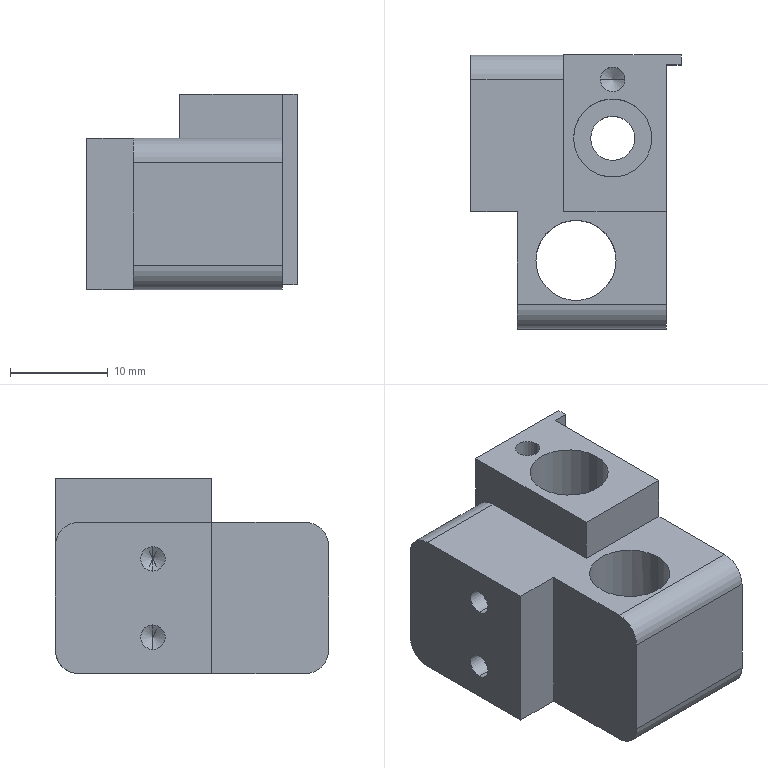Part | NX | features BREP 1 | 1 solid | 46 faces | box 21.5 x 28 x 20 mm | volume 6689 mm3 | cylinder 22 | plane 14 | cone 10 | commonest cylinder face diameters 2.5 x6 2.05 x4 5 x4 3.3 x2 4.5 x2 8 x2
STEP:
#1=CARTESIAN_POINT('',(20.,-9.5,15.5));
#2=VERTEX_POINT('',#1);
#3=CARTESIAN_POINT('',(20.,-12.,13.));
#4=VERTEX_POINT('',#3);
#5=CARTESIAN_POINT('',(20.,-9.5,13.));
#6=DIRECTION('',(1.,0.,0.));
#7=DIRECTION('',(0.,-1.,0.));
#8=AXIS2_PLACEMENT_3D('',#5,#6,#7);
#9=CIRCLE('',#8,2.5);
#10=EDGE_CURVE('',#2,#4,#9,.T.);
#11=ORIENTED_EDGE('',*,*,#10,.F.);
#12=CARTESIAN_POINT('',(4.75,-9.5,15.5));
#13=VERTEX_POINT('',#12);
#14=CARTESIAN_POINT('',(20.,-9.5,15.5));
#15=DIRECTION('',(1.,0.,0.));
#16=VECTOR('',#15,1000.);
#17=LINE('',#14,#16);
#18=EDGE_CURVE('',#13,#2,#17,.T.);
#19=ORIENTED_EDGE('',*,*,#18,.F.);
#20=CARTESIAN_POINT('',(4.75,-12.,13.));
#21=VERTEX_POINT('',#20);
#22=CARTESIAN_POINT('',(4.75,-9.5,13.));
#23=DIRECTION('',(-1.,0.,0.));
#24=DIRECTION('',(0.,0.,-1.));
#25=AXIS2_PLACEMENT_3D('',#22,#23,#24);
#26=CIRCLE('',#25,2.5);
#27=EDGE_CURVE('',#21,#13,#26,.T.);
#28=ORIENTED_EDGE('',*,*,#27,.F.);
#29=CARTESIAN_POINT('',(4.75,-12.,13.));
#30=DIRECTION('',(-1.,0.,0.));
#31=VECTOR('',#30,1000.);
#32=LINE('',#29,#31);
#33=EDGE_CURVE('',#4,#21,#32,.T.);
#34=ORIENTED_EDGE('',*,*,#33,.F.);
#35=EDGE_LOOP('',(#11,#19,#28,#34));
#36=FACE_BOUND('',#35,.T.);
#37=CARTESIAN_POINT('',(0.,-9.5,13.));
#38=DIRECTION('',(1.,0.,0.));
#39=DIRECTION('',(0.,1.,0.));
#40=AXIS2_PLACEMENT_3D('',#37,#38,#39);
#41=CYLINDRICAL_SURFACE('',#40,2.5);
#42=ADVANCED_FACE('',(#36),#41,.T.);
#43=CARTESIAN_POINT('',(4.75,-9.5,0.));
#44=VERTEX_POINT('',#43);
#45=CARTESIAN_POINT('',(4.75,-12.,2.5));
#46=VERTEX_POINT('',#45);
#47=CARTESIAN_POINT('',(4.75,-9.5,2.5));
#48=DIRECTION('',(-1.,0.,0.));
#49=DIRECTION('',(0.,0.,-1.));
#50=AXIS2_PLACEMENT_3D('',#47,#48,#49);
#51=CIRCLE('',#50,2.5);
#52=EDGE_CURVE('',#44,#46,#51,.T.);
#53=ORIENTED_EDGE('',*,*,#52,.F.);
#54=CARTESIAN_POINT('',(20.,-9.5,0.));
#55=VERTEX_POINT('',#54);
#56=CARTESIAN_POINT('',(0.,-9.5,0.));
#57=DIRECTION('',(-1.,0.,0.));
#58=VECTOR('',#57,1000.);
#59=LINE('',#56,#58);
#60=EDGE_CURVE('',#55,#44,#59,.T.);
#61=ORIENTED_EDGE('',*,*,#60,.F.);
#62=CARTESIAN_POINT('',(20.,-12.,2.5));
#63=VERTEX_POINT('',#62);
#64=CARTESIAN_POINT('',(20.,-9.5,2.5));
#65=DIRECTION('',(1.,0.,0.));
#66=DIRECTION('',(0.,-1.,0.));
#67=AXIS2_PLACEMENT_3D('',#64,#65,#66);
#68=CIRCLE('',#67,2.5);
#69=EDGE_CURVE('',#63,#55,#68,.T.);
#70=ORIENTED_EDGE('',*,*,#69,.F.);
#71=CARTESIAN_POINT('',(0.,-12.,2.5));
#72=DIRECTION('',(1.,0.,0.));
#73=VECTOR('',#72,1000.);
#74=LINE('',#71,#73);
#75=EDGE_CURVE('',#46,#63,#74,.T.);
#76=ORIENTED_EDGE('',*,*,#75,.F.);
#77=EDGE_LOOP('',(#53,#61,#70,#76));
#78=FACE_BOUND('',#77,.T.);
#79=CARTESIAN_POINT('',(0.,-9.5,2.5));
#80=DIRECTION('',(1.,0.,0.));
#81=DIRECTION('',(0.,1.,0.));
#82=AXIS2_PLACEMENT_3D('',#79,#80,#81);
#83=CYLINDRICAL_SURFACE('',#82,2.5);
#84=ADVANCED_FACE('',(#78),#83,.T.);
#85=CARTESIAN_POINT('',(14.85,-5.,9.65));
#86=VERTEX_POINT('',#85);
#87=CARTESIAN_POINT('',(20.,-5.,9.65));
#88=VERTEX_POINT('',#87);
#89=CARTESIAN_POINT('',(20.,-5.,9.65));
#90=DIRECTION('',(1.,0.,0.));
#91=VECTOR('',#90,1000.);
#92=LINE('',#89,#91);
#93=EDGE_CURVE('',#86,#88,#92,.T.);
#94=ORIENTED_EDGE('',*,*,#93,.F.);
#95=CARTESIAN_POINT('',(14.85,-5.,6.35));
#96=VERTEX_POINT('',#95);
#97=CARTESIAN_POINT('',(14.85,-5.,9.65));
#98=CARTESIAN_POINT('',(14.85,-4.793,9.65));
#99=CARTESIAN_POINT('',(14.815,-4.417,9.563));
#100=CARTESIAN_POINT('',(14.759,-4.135,9.414));
#101=CARTESIAN_POINT('',(14.697,-3.881,9.229));
#102=CARTESIAN_POINT('',(14.635,-3.689,9.006));
#103=CARTESIAN_POINT('',(14.609,-3.615,8.902));
#104=CARTESIAN_POINT('',(14.529,-3.402,8.528));
#105=CARTESIAN_POINT('',(14.486,-3.315,7.999));
#106=CARTESIAN_POINT('',(14.529,-3.403,7.471));
#107=CARTESIAN_POINT('',(14.609,-3.614,7.099));
#108=CARTESIAN_POINT('',(14.636,-3.69,6.992));
#109=CARTESIAN_POINT('',(14.696,-3.878,6.774));
#110=CARTESIAN_POINT('',(14.759,-4.135,6.586));
#111=CARTESIAN_POINT('',(14.815,-4.415,6.438));
#112=CARTESIAN_POINT('',(14.85,-4.793,6.35));
#113=CARTESIAN_POINT('',(14.85,-5.,6.35));
#114=B_SPLINE_CURVE_WITH_KNOTS('',3,(#97,#98,#99,#100,#101,#102,#103,#104,#105,#106,#107,#108,#109,#110,#111,#112,#113),.UNSPECIFIED.,.F.,.F.,(4,1,1,1,1,1,1,1,1,1,1,1,1,1,4),(0.,0.125,0.1875,0.25,0.2812,0.3125,0.375,0.5,0.625,0.6875,0.7188,0.75,0.8125,0.875,1.),.UNSPECIFIED.);
#115=EDGE_CURVE('',#96,#86,#114,.F.);
#116=ORIENTED_EDGE('',*,*,#115,.F.);
#117=CARTESIAN_POINT('',(20.,-5.,6.35));
#118=VERTEX_POINT('',#117);
#119=CARTESIAN_POINT('',(20.,-5.,6.35));
#120=DIRECTION('',(1.,0.,0.));
#121=VECTOR('',#120,1000.);
#122=LINE('',#119,#121);
#123=EDGE_CURVE('',#96,#118,#122,.T.);
#124=ORIENTED_EDGE('',*,*,#123,.T.);
#125=CARTESIAN_POINT('',(20.,-5.,8.));
#126=DIRECTION('',(1.,0.,0.));
#127=DIRECTION('',(0.,0.,-1.));
#128=AXIS2_PLACEMENT_3D('',#125,#126,#127);
#129=CIRCLE('',#128,1.65);
#130=EDGE_CURVE('',#118,#88,#129,.T.);
#131=ORIENTED_EDGE('',*,*,#130,.T.);
#132=EDGE_LOOP('',(#94,#116,#124,#131));
#133=FACE_BOUND('',#132,.T.);
#134=CARTESIAN_POINT('',(20.,-5.,8.));
#135=DIRECTION('',(1.,0.,0.));
#136=DIRECTION('',(0.,0.,-1.));
#137=AXIS2_PLACEMENT_3D('',#134,#135,#136);
#138=CYLINDRICAL_SURFACE('',#137,1.65);
#139=ADVANCED_FACE('',(#133),#138,.F.);
#140=CARTESIAN_POINT('',(6.65,-5.,15.5));
#141=VERTEX_POINT('',#140);
#142=CARTESIAN_POINT('',(6.65,-5.,0.));
#143=VERTEX_POINT('',#142);
#144=CARTESIAN_POINT('',(6.65,-5.,15.5));
#145=DIRECTION('',(0.,0.,1.));
#146=VECTOR('',#145,1000.);
#147=LINE('',#144,#146);
#148=EDGE_CURVE('',#141,#143,#147,.F.);
#149=ORIENTED_EDGE('',*,*,#148,.T.);
#150=CARTESIAN_POINT('',(14.85,-5.,0.));
#151=VERTEX_POINT('',#150);
#152=CARTESIAN_POINT('',(10.75,-5.,0.));
#153=DIRECTION('',(0.,0.,1.));
#154=DIRECTION('',(1.,0.,0.));
#155=AXIS2_PLACEMENT_3D('',#152,#153,#154);
#156=CIRCLE('',#155,4.1);
#157=EDGE_CURVE('',#151,#143,#156,.T.);
#158=ORIENTED_EDGE('',*,*,#157,.F.);
#159=CARTESIAN_POINT('',(14.85,-5.,15.5));
#160=DIRECTION('',(0.,0.,1.));
#161=VECTOR('',#160,1000.);
#162=LINE('',#159,#161);
#163=EDGE_CURVE('',#151,#96,#162,.T.);
#164=ORIENTED_EDGE('',*,*,#163,.T.);
#165=ORIENTED_EDGE('',*,*,#115,.T.);
#166=CARTESIAN_POINT('',(14.85,-5.,15.5));
#167=VERTEX_POINT('',#166);
#168=CARTESIAN_POINT('',(14.85,-5.,15.5));
#169=DIRECTION('',(0.,0.,1.));
#170=VECTOR('',#169,1000.);
#171=LINE('',#168,#170);
#172=EDGE_CURVE('',#167,#86,#171,.F.);
#173=ORIENTED_EDGE('',*,*,#172,.F.);
#174=CARTESIAN_POINT('',(10.75,-5.,15.5));
#175=DIRECTION('',(0.,0.,1.));
#176=DIRECTION('',(1.,0.,0.));
#177=AXIS2_PLACEMENT_3D('',#174,#175,#176);
#178=CIRCLE('',#177,4.1);
#179=EDGE_CURVE('',#167,#141,#178,.T.);
#180=ORIENTED_EDGE('',*,*,#179,.T.);
#181=EDGE_LOOP('',(#149,#158,#164,#165,#173,#180));
#182=FACE_BOUND('',#181,.T.);
#183=CARTESIAN_POINT('',(10.75,-5.,15.5));
#184=DIRECTION('',(0.,0.,1.));
#185=DIRECTION('',(1.,0.,0.));
#186=AXIS2_PLACEMENT_3D('',#183,#184,#185);
#187=CYLINDRICAL_SURFACE('',#186,4.1);
#188=ADVANCED_FACE('',(#182),#187,.F.);
#189=CARTESIAN_POINT('',(4.75,-12.,0.));
#190=DIRECTION('',(0.,0.,-1.));
#191=VECTOR('',#190,1000.);
#192=LINE('',#189,#191);
#193=EDGE_CURVE('',#21,#46,#192,.T.);
#194=ORIENTED_EDGE('',*,*,#193,.T.);
#195=ORIENTED_EDGE('',*,*,#75,.T.);
#196=CARTESIAN_POINT('',(20.,-12.,0.));
#197=DIRECTION('',(0.,0.,1.));
#198=VECTOR('',#197,1000.);
#199=LINE('',#196,#198);
#200=EDGE_CURVE('',#63,#4,#199,.T.);
#201=ORIENTED_EDGE('',*,*,#200,.T.);
#202=ORIENTED_EDGE('',*,*,#33,.T.);
#203=EDGE_LOOP('',(#194,#195,#201,#202));
#204=FACE_BOUND('',#203,.T.);
#205=CARTESIAN_POINT('',(0.,-12.,0.));
#206=DIRECTION('',(0.,-1.,0.));
#207=DIRECTION('',(1.,0.,0.));
#208=AXIS2_PLACEMENT_3D('',#205,#206,#207);
#209=PLANE('',#208);
#210=ADVANCED_FACE('',(#204),#209,.T.);
#211=CARTESIAN_POINT('',(4.75,0.,0.));
#212=VERTEX_POINT('',#211);
#213=CARTESIAN_POINT('',(4.75,-12.,0.));
#214=DIRECTION('',(0.,1.,0.));
#215=VECTOR('',#214,1000.);
#216=LINE('',#213,#215);
#217=EDGE_CURVE('',#44,#212,#216,.T.);
#218=ORIENTED_EDGE('',*,*,#217,.F.);
#219=ORIENTED_EDGE('',*,*,#52,.T.);
#220=ORIENTED_EDGE('',*,*,#193,.F.);
#221=ORIENTED_EDGE('',*,*,#27,.T.);
#222=CARTESIAN_POINT('',(4.75,0.,15.5));
#223=VERTEX_POINT('',#222);
#224=CARTESIAN_POINT('',(4.75,-12.,15.5));
#225=DIRECTION('',(0.,1.,0.));
#226=VECTOR('',#225,1000.);
#227=LINE('',#224,#226);
#228=EDGE_CURVE('',#13,#223,#227,.T.);
#229=ORIENTED_EDGE('',*,*,#228,.T.);
#230=CARTESIAN_POINT('',(4.75,0.,0.));
#231=DIRECTION('',(0.,0.,-1.));
#232=VECTOR('',#231,1000.);
#233=LINE('',#230,#232);
#234=EDGE_CURVE('',#223,#212,#233,.T.);
#235=ORIENTED_EDGE('',*,*,#234,.T.);
#236=EDGE_LOOP('',(#218,#219,#220,#221,#229,#235));
#237=FACE_BOUND('',#236,.T.);
#238=CARTESIAN_POINT('',(4.75,-12.,0.));
#239=DIRECTION('',(1.,0.,0.));
#240=DIRECTION('',(0.,0.,-1.));
#241=AXIS2_PLACEMENT_3D('',#238,#239,#240);
#242=PLANE('',#241);
#243=ADVANCED_FACE('',(#237),#242,.F.);
#244=CARTESIAN_POINT('',(9.5,16.,13.));
#245=VERTEX_POINT('',#244);
#246=CARTESIAN_POINT('',(9.5,13.5,15.5));
#247=VERTEX_POINT('',#246);
#248=CARTESIAN_POINT('',(9.5,13.5,13.));
#249=DIRECTION('',(1.,0.,0.));
#250=DIRECTION('',(0.,0.,-1.));
#251=AXIS2_PLACEMENT_3D('',#248,#249,#250);
#252=CIRCLE('',#251,2.5);
#253=EDGE_CURVE('',#245,#247,#252,.T.);
#254=ORIENTED_EDGE('',*,*,#253,.F.);
#255=CARTESIAN_POINT('',(0.,16.,13.));
#256=VERTEX_POINT('',#255);
#257=CARTESIAN_POINT('',(0.,16.,13.));
#258=DIRECTION('',(1.,0.,0.));
#259=VECTOR('',#258,1000.);
#260=LINE('',#257,#259);
#261=EDGE_CURVE('',#256,#245,#260,.T.);
#262=ORIENTED_EDGE('',*,*,#261,.F.);
#263=CARTESIAN_POINT('',(0.,13.5,15.5));
#264=VERTEX_POINT('',#263);
#265=CARTESIAN_POINT('',(0.,13.5,13.));
#266=DIRECTION('',(-1.,0.,0.));
#267=DIRECTION('',(0.,0.,-1.));
#268=AXIS2_PLACEMENT_3D('',#265,#266,#267);
#269=CIRCLE('',#268,2.5);
#270=EDGE_CURVE('',#264,#256,#269,.T.);
#271=ORIENTED_EDGE('',*,*,#270,.F.);
#272=CARTESIAN_POINT('',(0.,13.5,15.5));
#273=DIRECTION('',(-1.,0.,0.));
#274=VECTOR('',#273,1000.);
#275=LINE('',#272,#274);
#276=EDGE_CURVE('',#247,#264,#275,.T.);
#277=ORIENTED_EDGE('',*,*,#276,.F.);
#278=EDGE_LOOP('',(#254,#262,#271,#277));
#279=FACE_BOUND('',#278,.T.);
#280=CARTESIAN_POINT('',(0.,13.5,13.));
#281=DIRECTION('',(-1.,0.,0.));
#282=DIRECTION('',(0.,0.,1.));
#283=AXIS2_PLACEMENT_3D('',#280,#281,#282);
#284=CYLINDRICAL_SURFACE('',#283,2.5);
#285=ADVANCED_FACE('',(#279),#284,.T.);
#286=CARTESIAN_POINT('',(20.,13.5,0.));
#287=VERTEX_POINT('',#286);
#288=CARTESIAN_POINT('',(20.,15.,0.5));
#289=VERTEX_POINT('',#288);
#290=CARTESIAN_POINT('',(20.,13.5,2.5));
#291=DIRECTION('',(1.,0.,0.));
#292=DIRECTION('',(0.,-1.,0.));
#293=AXIS2_PLACEMENT_3D('',#290,#291,#292);
#294=CIRCLE('',#293,2.5);
#295=EDGE_CURVE('',#287,#289,#294,.T.);
#296=ORIENTED_EDGE('',*,*,#295,.F.);
#297=CARTESIAN_POINT('',(0.,13.5,0.));
#298=VERTEX_POINT('',#297);
#299=CARTESIAN_POINT('',(21.5,13.5,0.));
#300=DIRECTION('',(1.,0.,0.));
#301=VECTOR('',#300,1000.);
#302=LINE('',#299,#301);
#303=EDGE_CURVE('',#298,#287,#302,.T.);
#304=ORIENTED_EDGE('',*,*,#303,.F.);
#305=CARTESIAN_POINT('',(0.,16.,2.5));
#306=VERTEX_POINT('',#305);
#307=CARTESIAN_POINT('',(0.,13.5,2.5));
#308=DIRECTION('',(-1.,0.,0.));
#309=DIRECTION('',(0.,0.,-1.));
#310=AXIS2_PLACEMENT_3D('',#307,#308,#309);
#311=CIRCLE('',#310,2.5);
#312=EDGE_CURVE('',#306,#298,#311,.T.);
#313=ORIENTED_EDGE('',*,*,#312,.F.);
#314=CARTESIAN_POINT('',(21.5,16.,2.5));
#315=VERTEX_POINT('',#314);
#316=CARTESIAN_POINT('',(0.,16.,2.5));
#317=DIRECTION('',(-1.,0.,0.));
#318=VECTOR('',#317,1000.);
#319=LINE('',#316,#318);
#320=EDGE_CURVE('',#315,#306,#319,.T.);
#321=ORIENTED_EDGE('',*,*,#320,.F.);
#322=CARTESIAN_POINT('',(21.5,15.,0.5));
#323=VERTEX_POINT('',#322);
#324=CARTESIAN_POINT('',(21.5,13.5,2.5));
#325=DIRECTION('',(1.,0.,0.));
#326=DIRECTION('',(0.,0.,1.));
#327=AXIS2_PLACEMENT_3D('',#324,#325,#326);
#328=CIRCLE('',#327,2.5);
#329=EDGE_CURVE('',#323,#315,#328,.T.);
#330=ORIENTED_EDGE('',*,*,#329,.F.);
#331=CARTESIAN_POINT('',(20.,15.,0.5));
#332=DIRECTION('',(1.,0.,0.));
#333=VECTOR('',#332,1000.);
#334=LINE('',#331,#333);
#335=EDGE_CURVE('',#289,#323,#334,.T.);
#336=ORIENTED_EDGE('',*,*,#335,.F.);
#337=EDGE_LOOP('',(#296,#304,#313,#321,#330,#336));
#338=FACE_BOUND('',#337,.T.);
#339=CARTESIAN_POINT('',(0.,13.5,2.5));
#340=DIRECTION('',(1.,0.,0.));
#341=DIRECTION('',(0.,0.,-1.));
#342=AXIS2_PLACEMENT_3D('',#339,#340,#341);
#343=CYLINDRICAL_SURFACE('',#342,2.5);
#344=ADVANCED_FACE('',(#338),#343,.T.);
#345=ORIENTED_EDGE('',*,*,#228,.F.);
#346=ORIENTED_EDGE('',*,*,#18,.T.);
#347=CARTESIAN_POINT('',(20.,0.,15.5));
#348=VERTEX_POINT('',#347);
#349=CARTESIAN_POINT('',(20.,-12.,15.5));
#350=DIRECTION('',(0.,1.,0.));
#351=VECTOR('',#350,1000.);
#352=LINE('',#349,#351);
#353=EDGE_CURVE('',#2,#348,#352,.T.);
#354=ORIENTED_EDGE('',*,*,#353,.T.);
#355=CARTESIAN_POINT('',(9.5,0.,15.5));
#356=VERTEX_POINT('',#355);
#357=CARTESIAN_POINT('',(20.,0.,15.5));
#358=DIRECTION('',(-1.,0.,0.));
#359=VECTOR('',#358,1000.);
#360=LINE('',#357,#359);
#361=EDGE_CURVE('',#348,#356,#360,.T.);
#362=ORIENTED_EDGE('',*,*,#361,.T.);
#363=CARTESIAN_POINT('',(9.5,0.,15.5));
#364=DIRECTION('',(0.,1.,0.));
#365=VECTOR('',#364,1000.);
#366=LINE('',#363,#365);
#367=EDGE_CURVE('',#356,#247,#366,.T.);
#368=ORIENTED_EDGE('',*,*,#367,.T.);
#369=ORIENTED_EDGE('',*,*,#276,.T.);
#370=CARTESIAN_POINT('',(0.,0.,15.5));
#371=VERTEX_POINT('',#370);
#372=CARTESIAN_POINT('',(0.,0.,15.5));
#373=DIRECTION('',(0.,-1.,0.));
#374=VECTOR('',#373,1000.);
#375=LINE('',#372,#374);
#376=EDGE_CURVE('',#264,#371,#375,.T.);
#377=ORIENTED_EDGE('',*,*,#376,.T.);
#378=CARTESIAN_POINT('',(0.,0.,15.5));
#379=DIRECTION('',(1.,0.,0.));
#380=VECTOR('',#379,1000.);
#381=LINE('',#378,#380);
#382=EDGE_CURVE('',#371,#223,#381,.T.);
#383=ORIENTED_EDGE('',*,*,#382,.T.);
#384=EDGE_LOOP('',(#345,#346,#354,#362,#368,#369,#377,#383));
#385=FACE_BOUND('',#384,.T.);
#386=ORIENTED_EDGE('',*,*,#179,.F.);
#387=CARTESIAN_POINT('',(10.75,-5.,15.5));
#388=DIRECTION('',(0.,0.,1.));
#389=DIRECTION('',(1.,0.,0.));
#390=AXIS2_PLACEMENT_3D('',#387,#388,#389);
#391=CIRCLE('',#390,4.1);
#392=EDGE_CURVE('',#141,#167,#391,.T.);
#393=ORIENTED_EDGE('',*,*,#392,.F.);
#394=EDGE_LOOP('',(#386,#393));
#395=FACE_BOUND('',#394,.T.);
#396=CARTESIAN_POINT('',(0.,0.,15.5));
#397=DIRECTION('',(0.,0.,-1.));
#398=DIRECTION('',(-1.,0.,0.));
#399=AXIS2_PLACEMENT_3D('',#396,#397,#398);
#400=PLANE('',#399);
#401=ADVANCED_FACE('',(#385,#395),#400,.F.);
#402=CARTESIAN_POINT('',(9.5,0.,20.));
#403=VERTEX_POINT('',#402);
#404=CARTESIAN_POINT('',(9.5,16.,20.));
#405=VERTEX_POINT('',#404);
#406=CARTESIAN_POINT('',(9.5,0.,20.));
#407=DIRECTION('',(0.,1.,0.));
#408=VECTOR('',#407,1000.);
#409=LINE('',#406,#408);
#410=EDGE_CURVE('',#403,#405,#409,.T.);
#411=ORIENTED_EDGE('',*,*,#410,.T.);
#412=CARTESIAN_POINT('',(9.5,16.,15.5));
#413=DIRECTION('',(0.,0.,1.));
#414=VECTOR('',#413,1000.);
#415=LINE('',#412,#414);
#416=EDGE_CURVE('',#245,#405,#415,.T.);
#417=ORIENTED_EDGE('',*,*,#416,.F.);
#418=ORIENTED_EDGE('',*,*,#253,.T.);
#419=ORIENTED_EDGE('',*,*,#367,.F.);
#420=CARTESIAN_POINT('',(9.5,0.,15.5));
#421=DIRECTION('',(0.,0.,1.));
#422=VECTOR('',#421,1000.);
#423=LINE('',#420,#422);
#424=EDGE_CURVE('',#356,#403,#423,.T.);
#425=ORIENTED_EDGE('',*,*,#424,.T.);
#426=EDGE_LOOP('',(#411,#417,#418,#419,#425));
#427=FACE_BOUND('',#426,.T.);
#428=CARTESIAN_POINT('',(9.5,0.,15.5));
#429=DIRECTION('',(1.,0.,0.));
#430=DIRECTION('',(0.,0.,-1.));
#431=AXIS2_PLACEMENT_3D('',#428,#429,#430);
#432=PLANE('',#431);
#433=ADVANCED_FACE('',(#427),#432,.F.);
#434=CARTESIAN_POINT('',(0.,6.,2.5));
#435=VERTEX_POINT('',#434);
#436=CARTESIAN_POINT('',(9.5,6.,2.5));
#437=VERTEX_POINT('',#436);
#438=CARTESIAN_POINT('',(0.,6.,2.5));
#439=DIRECTION('',(-1.,0.,0.));
#440=VECTOR('',#439,1000.);
#441=LINE('',#438,#440);
#442=EDGE_CURVE('',#435,#437,#441,.F.);
#443=ORIENTED_EDGE('',*,*,#442,.T.);
#444=CARTESIAN_POINT('',(9.5,6.,5.));
#445=VERTEX_POINT('',#444);
#446=CARTESIAN_POINT('',(9.5,6.,3.75));
#447=DIRECTION('',(-1.,0.,0.));
#448=DIRECTION('',(0.,0.,1.));
#449=AXIS2_PLACEMENT_3D('',#446,#447,#448);
#450=CIRCLE('',#449,1.25);
#451=EDGE_CURVE('',#445,#437,#450,.T.);
#452=ORIENTED_EDGE('',*,*,#451,.F.);
#453=CARTESIAN_POINT('',(0.,6.,5.));
#454=VERTEX_POINT('',#453);
#455=CARTESIAN_POINT('',(0.,6.,5.));
#456=DIRECTION('',(-1.,0.,0.));
#457=VECTOR('',#456,1000.);
#458=LINE('',#455,#457);
#459=EDGE_CURVE('',#454,#445,#458,.F.);
#460=ORIENTED_EDGE('',*,*,#459,.F.);
#461=CARTESIAN_POINT('',(0.,6.,3.75));
#462=DIRECTION('',(-1.,0.,0.));
#463=DIRECTION('',(0.,0.,1.));
#464=AXIS2_PLACEMENT_3D('',#461,#462,#463);
#465=CIRCLE('',#464,1.25);
#466=EDGE_CURVE('',#454,#435,#465,.T.);
#467=ORIENTED_EDGE('',*,*,#466,.T.);
#468=EDGE_LOOP('',(#443,#452,#460,#467));
#469=FACE_BOUND('',#468,.T.);
#470=CARTESIAN_POINT('',(0.,6.,3.75));
#471=DIRECTION('',(-1.,0.,0.));
#472=DIRECTION('',(0.,0.,1.));
#473=AXIS2_PLACEMENT_3D('',#470,#471,#472);
#474=CYLINDRICAL_SURFACE('',#473,1.25);
#475=ADVANCED_FACE('',(#469),#474,.F.);
#476=CARTESIAN_POINT('',(10.251,6.,3.75));
#477=VERTEX_POINT('',#476);
#478=CARTESIAN_POINT('',(9.5,6.,2.5));
#479=DIRECTION('',(-0.515,0.,-0.8572));
#480=VECTOR('',#479,1000.);
#481=LINE('',#478,#480);
#482=EDGE_CURVE('',#477,#437,#481,.T.);
#483=ORIENTED_EDGE('',*,*,#482,.F.);
#484=CARTESIAN_POINT('',(9.5,6.,5.));
#485=DIRECTION('',(-0.515,0.,0.8572));
#486=VECTOR('',#485,1000.);
#487=LINE('',#484,#486);
#488=EDGE_CURVE('',#477,#445,#487,.T.);
#489=ORIENTED_EDGE('',*,*,#488,.T.);
#490=ORIENTED_EDGE('',*,*,#451,.T.);
#491=EDGE_LOOP('',(#483,#489,#490));
#492=FACE_BOUND('',#491,.T.);
#493=CARTESIAN_POINT('',(9.5,6.,3.75));
#494=DIRECTION('',(-1.,0.,0.));
#495=DIRECTION('',(0.,0.,1.));
#496=AXIS2_PLACEMENT_3D('',#493,#494,#495);
#497=CONICAL_SURFACE('',#496,1.25,1.03);
#498=ADVANCED_FACE('',(#492),#497,.F.);
#499=CARTESIAN_POINT('',(0.,6.,10.5));
#500=VERTEX_POINT('',#499);
#501=CARTESIAN_POINT('',(9.5,6.,10.5));
#502=VERTEX_POINT('',#501);
#503=CARTESIAN_POINT('',(0.,6.,10.5));
#504=DIRECTION('',(-1.,0.,0.));
#505=VECTOR('',#504,1000.);
#506=LINE('',#503,#505);
#507=EDGE_CURVE('',#500,#502,#506,.F.);
#508=ORIENTED_EDGE('',*,*,#507,.T.);
#509=CARTESIAN_POINT('',(9.5,6.,13.));
#510=VERTEX_POINT('',#509);
#511=CARTESIAN_POINT('',(9.5,6.,11.75));
#512=DIRECTION('',(-1.,0.,0.));
#513=DIRECTION('',(0.,0.,1.));
#514=AXIS2_PLACEMENT_3D('',#511,#512,#513);
#515=CIRCLE('',#514,1.25);
#516=EDGE_CURVE('',#510,#502,#515,.T.);
#517=ORIENTED_EDGE('',*,*,#516,.F.);
#518=CARTESIAN_POINT('',(0.,6.,13.));
#519=VERTEX_POINT('',#518);
#520=CARTESIAN_POINT('',(0.,6.,13.));
#521=DIRECTION('',(-1.,0.,0.));
#522=VECTOR('',#521,1000.);
#523=LINE('',#520,#522);
#524=EDGE_CURVE('',#519,#510,#523,.F.);
#525=ORIENTED_EDGE('',*,*,#524,.F.);
#526=CARTESIAN_POINT('',(0.,6.,11.75));
#527=DIRECTION('',(-1.,0.,0.));
#528=DIRECTION('',(0.,0.,1.));
#529=AXIS2_PLACEMENT_3D('',#526,#527,#528);
#530=CIRCLE('',#529,1.25);
#531=EDGE_CURVE('',#519,#500,#530,.T.);
#532=ORIENTED_EDGE('',*,*,#531,.T.);
#533=EDGE_LOOP('',(#508,#517,#525,#532));
#534=FACE_BOUND('',#533,.T.);
#535=CARTESIAN_POINT('',(0.,6.,11.75));
#536=DIRECTION('',(-1.,0.,0.));
#537=DIRECTION('',(0.,0.,1.));
#538=AXIS2_PLACEMENT_3D('',#535,#536,#537);
#539=CYLINDRICAL_SURFACE('',#538,1.25);
#540=ADVANCED_FACE('',(#534),#539,.F.);
#541=CARTESIAN_POINT('',(10.251,6.,11.75));
#542=VERTEX_POINT('',#541);
#543=CARTESIAN_POINT('',(9.5,6.,10.5));
#544=DIRECTION('',(-0.515,0.,-0.8572));
#545=VECTOR('',#544,1000.);
#546=LINE('',#543,#545);
#547=EDGE_CURVE('',#542,#502,#546,.T.);
#548=ORIENTED_EDGE('',*,*,#547,.F.);
#549=CARTESIAN_POINT('',(9.5,6.,13.));
#550=DIRECTION('',(-0.515,0.,0.8572));
#551=VECTOR('',#550,1000.);
#552=LINE('',#549,#551);
#553=EDGE_CURVE('',#542,#510,#552,.T.);
#554=ORIENTED_EDGE('',*,*,#553,.T.);
#555=ORIENTED_EDGE('',*,*,#516,.T.);
#556=EDGE_LOOP('',(#548,#554,#555));
#557=FACE_BOUND('',#556,.T.);
#558=CARTESIAN_POINT('',(9.5,6.,11.75));
#559=DIRECTION('',(-1.,0.,0.));
#560=DIRECTION('',(0.,0.,1.));
#561=AXIS2_PLACEMENT_3D('',#558,#559,#560);
#562=CONICAL_SURFACE('',#561,1.25,1.03);
#563=ADVANCED_FACE('',(#557),#562,.F.);
#564=CARTESIAN_POINT('',(14.15,2.5,18.525));
#565=VERTEX_POINT('',#564);
#566=CARTESIAN_POINT('',(20.,2.5,18.525));
#567=VERTEX_POINT('',#566);
#568=CARTESIAN_POINT('',(21.5,2.5,18.525));
#569=DIRECTION('',(1.,0.,0.));
#570=VECTOR('',#569,1000.);
#571=LINE('',#568,#570);
#572=EDGE_CURVE('',#565,#567,#571,.T.);
#573=ORIENTED_EDGE('',*,*,#572,.F.);
#574=CARTESIAN_POINT('',(14.15,3.515,17.64));
#575=VERTEX_POINT('',#574);
#576=CARTESIAN_POINT('',(14.15,2.5,17.5));
#577=DIRECTION('',(1.,0.,0.));
#578=DIRECTION('',(0.,0.,-1.));
#579=AXIS2_PLACEMENT_3D('',#576,#577,#578);
#580=CIRCLE('',#579,1.025);
#581=EDGE_CURVE('',#575,#565,#580,.T.);
#582=ORIENTED_EDGE('',*,*,#581,.F.);
#583=CARTESIAN_POINT('',(14.15,3.515,17.36));
#584=VERTEX_POINT('',#583);
#585=CARTESIAN_POINT('',(14.15,3.515,17.64));
#586=CARTESIAN_POINT('',(14.262,3.506,17.711));
#587=CARTESIAN_POINT('',(14.522,3.495,17.741));
#588=CARTESIAN_POINT('',(14.806,3.51,17.69));
#589=CARTESIAN_POINT('',(15.016,3.533,17.502));
#590=CARTESIAN_POINT('',(14.808,3.51,17.311));
#591=CARTESIAN_POINT('',(14.521,3.495,17.259));
#592=CARTESIAN_POINT('',(14.262,3.505,17.288));
#593=CARTESIAN_POINT('',(14.15,3.515,17.36));
#594=B_SPLINE_CURVE_WITH_KNOTS('',3,(#585,#586,#587,#588,#589,#590,#591,#592,#593),.UNSPECIFIED.,.F.,.F.,(4,1,1,1,1,1,4),(0.,0.25,0.375,0.5,0.625,0.75,1.),.UNSPECIFIED.);
#595=EDGE_CURVE('',#584,#575,#594,.F.);
#596=ORIENTED_EDGE('',*,*,#595,.F.);
#597=CARTESIAN_POINT('',(14.15,2.5,16.475));
#598=VERTEX_POINT('',#597);
#599=CARTESIAN_POINT('',(14.15,2.5,17.5));
#600=DIRECTION('',(1.,0.,0.));
#601=DIRECTION('',(0.,0.,-1.));
#602=AXIS2_PLACEMENT_3D('',#599,#600,#601);
#603=CIRCLE('',#602,1.025);
#604=EDGE_CURVE('',#598,#584,#603,.T.);
#605=ORIENTED_EDGE('',*,*,#604,.F.);
#606=CARTESIAN_POINT('',(20.,2.5,16.475));
#607=VERTEX_POINT('',#606);
#608=CARTESIAN_POINT('',(21.5,2.5,16.475));
#609=DIRECTION('',(1.,0.,0.));
#610=VECTOR('',#609,1000.);
#611=LINE('',#608,#610);
#612=EDGE_CURVE('',#598,#607,#611,.T.);
#613=ORIENTED_EDGE('',*,*,#612,.T.);
#614=CARTESIAN_POINT('',(20.,2.5,17.5));
#615=DIRECTION('',(-1.,0.,0.));
#616=DIRECTION('',(0.,-1.,0.));
#617=AXIS2_PLACEMENT_3D('',#614,#615,#616);
#618=CIRCLE('',#617,1.025);
#619=EDGE_CURVE('',#567,#607,#618,.T.);
#620=ORIENTED_EDGE('',*,*,#619,.F.);
#621=EDGE_LOOP('',(#573,#582,#596,#605,#613,#620));
#622=FACE_BOUND('',#621,.T.);
#623=CARTESIAN_POINT('',(21.5,2.5,17.5));
#624=DIRECTION('',(1.,0.,0.));
#625=DIRECTION('',(0.,0.,-1.));
#626=AXIS2_PLACEMENT_3D('',#623,#624,#625);
#627=CYLINDRICAL_SURFACE('',#626,1.025);
#628=ADVANCED_FACE('',(#622),#627,.F.);
#629=CARTESIAN_POINT('',(13.534,2.5,17.5));
#630=VERTEX_POINT('',#629);
#631=CARTESIAN_POINT('',(14.15,2.5,18.525));
#632=DIRECTION('',(0.515,0.,0.8572));
#633=VECTOR('',#632,1000.);
#634=LINE('',#631,#633);
#635=EDGE_CURVE('',#565,#630,#634,.F.);
#636=ORIENTED_EDGE('',*,*,#635,.T.);
#637=CARTESIAN_POINT('',(14.15,2.5,16.475));
#638=DIRECTION('',(0.515,0.,-0.8572));
#639=VECTOR('',#638,1000.);
#640=LINE('',#637,#639);
#641=EDGE_CURVE('',#598,#630,#640,.F.);
#642=ORIENTED_EDGE('',*,*,#641,.F.);
#643=ORIENTED_EDGE('',*,*,#604,.T.);
#644=CARTESIAN_POINT('',(14.15,3.515,17.64));
#645=CARTESIAN_POINT('',(14.143,3.516,17.547));
#646=CARTESIAN_POINT('',(14.143,3.516,17.453));
#647=CARTESIAN_POINT('',(14.15,3.515,17.36));
#648=B_SPLINE_CURVE_WITH_KNOTS('',3,(#644,#645,#646,#647),.UNSPECIFIED.,.F.,.F.,(4,4),(0.,1.),.UNSPECIFIED.);
#649=EDGE_CURVE('',#575,#584,#648,.T.);
#650=ORIENTED_EDGE('',*,*,#649,.F.);
#651=ORIENTED_EDGE('',*,*,#581,.T.);
#652=EDGE_LOOP('',(#636,#642,#643,#650,#651));
#653=FACE_BOUND('',#652,.T.);
#654=CARTESIAN_POINT('',(14.15,2.5,17.5));
#655=DIRECTION('',(1.,0.,0.));
#656=DIRECTION('',(0.,0.,-1.));
#657=AXIS2_PLACEMENT_3D('',#654,#655,#656);
#658=CONICAL_SURFACE('',#657,1.025,1.03);
#659=ADVANCED_FACE('',(#653),#658,.F.);
#660=CARTESIAN_POINT('',(14.15,2.5,5.025));
#661=VERTEX_POINT('',#660);
#662=CARTESIAN_POINT('',(13.534,2.5,4.));
#663=VERTEX_POINT('',#662);
#664=CARTESIAN_POINT('',(14.15,2.5,5.025));
#665=DIRECTION('',(0.515,0.,0.8572));
#666=VECTOR('',#665,1000.);
#667=LINE('',#664,#666);
#668=EDGE_CURVE('',#661,#663,#667,.F.);
#669=ORIENTED_EDGE('',*,*,#668,.T.);
#670=CARTESIAN_POINT('',(14.15,2.5,2.975));
#671=VERTEX_POINT('',#670);
#672=CARTESIAN_POINT('',(14.15,2.5,2.975));
#673=DIRECTION('',(0.515,0.,-0.8572));
#674=VECTOR('',#673,1000.);
#675=LINE('',#672,#674);
#676=EDGE_CURVE('',#671,#663,#675,.F.);
#677=ORIENTED_EDGE('',*,*,#676,.F.);
#678=CARTESIAN_POINT('',(14.15,2.5,4.));
#679=DIRECTION('',(1.,0.,0.));
#680=DIRECTION('',(0.,0.,-1.));
#681=AXIS2_PLACEMENT_3D('',#678,#679,#680);
#682=CIRCLE('',#681,1.025);
#683=EDGE_CURVE('',#671,#661,#682,.T.);
#684=ORIENTED_EDGE('',*,*,#683,.T.);
#685=EDGE_LOOP('',(#669,#677,#684));
#686=FACE_BOUND('',#685,.T.);
#687=CARTESIAN_POINT('',(14.15,2.5,4.));
#688=DIRECTION('',(1.,0.,0.));
#689=DIRECTION('',(0.,0.,-1.));
#690=AXIS2_PLACEMENT_3D('',#687,#688,#689);
#691=CONICAL_SURFACE('',#690,1.025,1.03);
#692=ADVANCED_FACE('',(#686),#691,.F.);
#693=CARTESIAN_POINT('',(20.,2.5,5.025));
#694=VERTEX_POINT('',#693);
#695=CARTESIAN_POINT('',(21.5,2.5,5.025));
#696=DIRECTION('',(1.,0.,0.));
#697=VECTOR('',#696,1000.);
#698=LINE('',#695,#697);
#699=EDGE_CURVE('',#661,#694,#698,.T.);
#700=ORIENTED_EDGE('',*,*,#699,.F.);
#701=ORIENTED_EDGE('',*,*,#683,.F.);
#702=CARTESIAN_POINT('',(20.,2.5,2.975));
#703=VERTEX_POINT('',#702);
#704=CARTESIAN_POINT('',(21.5,2.5,2.975));
#705=DIRECTION('',(1.,0.,0.));
#706=VECTOR('',#705,1000.);
#707=LINE('',#704,#706);
#708=EDGE_CURVE('',#671,#703,#707,.T.);
#709=ORIENTED_EDGE('',*,*,#708,.T.);
#710=CARTESIAN_POINT('',(20.,2.5,4.));
#711=DIRECTION('',(-1.,0.,0.));
#712=DIRECTION('',(0.,-1.,0.));
#713=AXIS2_PLACEMENT_3D('',#710,#711,#712);
#714=CIRCLE('',#713,1.025);
#715=EDGE_CURVE('',#694,#703,#714,.T.);
#716=ORIENTED_EDGE('',*,*,#715,.F.);
#717=EDGE_LOOP('',(#700,#701,#709,#716));
#718=FACE_BOUND('',#717,.T.);
#719=CARTESIAN_POINT('',(21.5,2.5,4.));
#720=DIRECTION('',(1.,0.,0.));
#721=DIRECTION('',(0.,0.,-1.));
#722=AXIS2_PLACEMENT_3D('',#719,#720,#721);
#723=CYLINDRICAL_SURFACE('',#722,1.025);
#724=ADVANCED_FACE('',(#718),#723,.F.);
#725=CARTESIAN_POINT('',(13.25,13.5,20.));
#726=VERTEX_POINT('',#725);
#727=CARTESIAN_POINT('',(13.25,13.5,10.5));
#728=VERTEX_POINT('',#727);
#729=CARTESIAN_POINT('',(13.25,13.5,20.));
#730=DIRECTION('',(0.,0.,1.));
#731=VECTOR('',#730,1000.);
#732=LINE('',#729,#731);
#733=EDGE_CURVE('',#726,#728,#732,.F.);
#734=ORIENTED_EDGE('',*,*,#733,.T.);
#735=CARTESIAN_POINT('',(15.75,13.5,10.5));
#736=VERTEX_POINT('',#735);
#737=CARTESIAN_POINT('',(14.5,13.5,10.5));
#738=DIRECTION('',(0.,0.,1.));
#739=DIRECTION('',(1.,0.,0.));
#740=AXIS2_PLACEMENT_3D('',#737,#738,#739);
#741=CIRCLE('',#740,1.25);
#742=EDGE_CURVE('',#736,#728,#741,.T.);
#743=ORIENTED_EDGE('',*,*,#742,.F.);
#744=CARTESIAN_POINT('',(15.75,13.5,20.));
#745=VERTEX_POINT('',#744);
#746=CARTESIAN_POINT('',(15.75,13.5,20.));
#747=DIRECTION('',(0.,0.,1.));
#748=VECTOR('',#747,1000.);
#749=LINE('',#746,#748);
#750=EDGE_CURVE('',#745,#736,#749,.F.);
#751=ORIENTED_EDGE('',*,*,#750,.F.);
#752=CARTESIAN_POINT('',(14.5,13.5,20.));
#753=DIRECTION('',(0.,0.,1.));
#754=DIRECTION('',(1.,0.,0.));
#755=AXIS2_PLACEMENT_3D('',#752,#753,#754);
#756=CIRCLE('',#755,1.25);
#757=EDGE_CURVE('',#745,#726,#756,.T.);
#758=ORIENTED_EDGE('',*,*,#757,.T.);
#759=EDGE_LOOP('',(#734,#743,#751,#758));
#760=FACE_BOUND('',#759,.T.);
#761=CARTESIAN_POINT('',(14.5,13.5,20.));
#762=DIRECTION('',(0.,0.,1.));
#763=DIRECTION('',(1.,0.,0.));
#764=AXIS2_PLACEMENT_3D('',#761,#762,#763);
#765=CYLINDRICAL_SURFACE('',#764,1.25);
#766=ADVANCED_FACE('',(#760),#765,.F.);
#767=CARTESIAN_POINT('',(14.5,13.5,9.749));
#768=VERTEX_POINT('',#767);
#769=CARTESIAN_POINT('',(13.25,13.5,10.5));
#770=DIRECTION('',(-0.8572,0.,0.515));
#771=VECTOR('',#770,1000.);
#772=LINE('',#769,#771);
#773=EDGE_CURVE('',#768,#728,#772,.T.);
#774=ORIENTED_EDGE('',*,*,#773,.F.);
#775=CARTESIAN_POINT('',(15.75,13.5,10.5));
#776=DIRECTION('',(0.8572,0.,0.515));
#777=VECTOR('',#776,1000.);
#778=LINE('',#775,#777);
#779=EDGE_CURVE('',#768,#736,#778,.T.);
#780=ORIENTED_EDGE('',*,*,#779,.T.);
#781=ORIENTED_EDGE('',*,*,#742,.T.);
#782=EDGE_LOOP('',(#774,#780,#781));
#783=FACE_BOUND('',#782,.T.);
#784=CARTESIAN_POINT('',(14.5,13.5,10.5));
#785=DIRECTION('',(0.,0.,1.));
#786=DIRECTION('',(1.,0.,0.));
#787=AXIS2_PLACEMENT_3D('',#784,#785,#786);
#788=CONICAL_SURFACE('',#787,1.25,1.03);
#789=ADVANCED_FACE('',(#783),#788,.F.);
#790=CARTESIAN_POINT('',(12.25,7.5,7.));
#791=VERTEX_POINT('',#790);
#792=CARTESIAN_POINT('',(12.25,7.5,0.));
#793=VERTEX_POINT('',#792);
#794=CARTESIAN_POINT('',(12.25,7.5,-12.));
#795=DIRECTION('',(0.,0.,1.));
#796=VECTOR('',#795,1000.);
#797=LINE('',#794,#796);
#798=EDGE_CURVE('',#791,#793,#797,.F.);
#799=ORIENTED_EDGE('',*,*,#798,.T.);
#800=CARTESIAN_POINT('',(16.75,7.5,0.));
#801=VERTEX_POINT('',#800);
#802=CARTESIAN_POINT('',(14.5,7.5,0.));
#803=DIRECTION('',(0.,0.,-1.));
#804=DIRECTION('',(-1.,0.,0.));
#805=AXIS2_PLACEMENT_3D('',#802,#803,#804);
#806=CIRCLE('',#805,2.25);
#807=EDGE_CURVE('',#793,#801,#806,.T.);
#808=ORIENTED_EDGE('',*,*,#807,.T.);
#809=CARTESIAN_POINT('',(16.75,7.5,7.));
#810=VERTEX_POINT('',#809);
#811=CARTESIAN_POINT('',(16.75,7.5,-12.));
#812=DIRECTION('',(0.,0.,1.));
#813=VECTOR('',#812,1000.);
#814=LINE('',#811,#813);
#815=EDGE_CURVE('',#810,#801,#814,.F.);
#816=ORIENTED_EDGE('',*,*,#815,.F.);
#817=CARTESIAN_POINT('',(14.5,7.5,7.));
#818=DIRECTION('',(0.,0.,1.));
#819=DIRECTION('',(1.,0.,0.));
#820=AXIS2_PLACEMENT_3D('',#817,#818,#819);
#821=CIRCLE('',#820,2.25);
#822=EDGE_CURVE('',#810,#791,#821,.T.);
#823=ORIENTED_EDGE('',*,*,#822,.T.);
#824=EDGE_LOOP('',(#799,#808,#816,#823));
#825=FACE_BOUND('',#824,.T.);
#826=CARTESIAN_POINT('',(14.5,7.5,-12.));
#827=DIRECTION('',(0.,0.,1.));
#828=DIRECTION('',(1.,0.,0.));
#829=AXIS2_PLACEMENT_3D('',#826,#827,#828);
#830=CYLINDRICAL_SURFACE('',#829,2.25);
#831=ADVANCED_FACE('',(#825),#830,.F.);
#832=CARTESIAN_POINT('',(18.5,7.5,7.));
#833=VERTEX_POINT('',#832);
#834=CARTESIAN_POINT('',(10.5,7.5,7.));
#835=VERTEX_POINT('',#834);
#836=CARTESIAN_POINT('',(14.5,7.5,7.));
#837=DIRECTION('',(0.,0.,1.));
#838=DIRECTION('',(1.,0.,0.));
#839=AXIS2_PLACEMENT_3D('',#836,#837,#838);
#840=CIRCLE('',#839,4.);
#841=EDGE_CURVE('',#833,#835,#840,.T.);
#842=ORIENTED_EDGE('',*,*,#841,.T.);
#843=CARTESIAN_POINT('',(14.5,7.5,7.));
#844=DIRECTION('',(0.,0.,1.));
#845=DIRECTION('',(1.,0.,0.));
#846=AXIS2_PLACEMENT_3D('',#843,#844,#845);
#847=CIRCLE('',#846,4.);
#848=EDGE_CURVE('',#835,#833,#847,.T.);
#849=ORIENTED_EDGE('',*,*,#848,.T.);
#850=EDGE_LOOP('',(#842,#849));
#851=FACE_BOUND('',#850,.T.);
#852=ORIENTED_EDGE('',*,*,#822,.F.);
#853=CARTESIAN_POINT('',(14.5,7.5,7.));
#854=DIRECTION('',(0.,0.,1.));
#855=DIRECTION('',(1.,0.,0.));
#856=AXIS2_PLACEMENT_3D('',#853,#854,#855);
#857=CIRCLE('',#856,2.25);
#858=EDGE_CURVE('',#791,#810,#857,.T.);
#859=ORIENTED_EDGE('',*,*,#858,.F.);
#860=EDGE_LOOP('',(#852,#859));
#861=FACE_BOUND('',#860,.T.);
#862=CARTESIAN_POINT('',(14.5,7.5,7.));
#863=DIRECTION('',(0.,0.,1.));
#864=DIRECTION('',(1.,0.,0.));
#865=AXIS2_PLACEMENT_3D('',#862,#863,#864);
#866=PLANE('',#865);
#867=ADVANCED_FACE('',(#851,#861),#866,.T.);
#868=CARTESIAN_POINT('',(10.5,7.5,20.));
#869=VERTEX_POINT('',#868);
#870=CARTESIAN_POINT('',(10.5,7.5,7.));
#871=DIRECTION('',(0.,0.,1.));
#872=VECTOR('',#871,1000.);
#873=LINE('',#870,#872);
#874=EDGE_CURVE('',#869,#835,#873,.F.);
#875=ORIENTED_EDGE('',*,*,#874,.T.);
#876=ORIENTED_EDGE('',*,*,#841,.F.);
#877=CARTESIAN_POINT('',(18.5,7.5,20.));
#878=VERTEX_POINT('',#877);
#879=CARTESIAN_POINT('',(18.5,7.5,7.));
#880=DIRECTION('',(0.,0.,1.));
#881=VECTOR('',#880,1000.);
#882=LINE('',#879,#881);
#883=EDGE_CURVE('',#878,#833,#882,.F.);
#884=ORIENTED_EDGE('',*,*,#883,.F.);
#885=CARTESIAN_POINT('',(14.5,7.5,20.));
#886=DIRECTION('',(0.,0.,1.));
#887=DIRECTION('',(1.,0.,0.));
#888=AXIS2_PLACEMENT_3D('',#885,#886,#887);
#889=CIRCLE('',#888,4.);
#890=EDGE_CURVE('',#878,#869,#889,.T.);
#891=ORIENTED_EDGE('',*,*,#890,.T.);
#892=EDGE_LOOP('',(#875,#876,#884,#891));
#893=FACE_BOUND('',#892,.T.);
#894=CARTESIAN_POINT('',(14.5,7.5,7.));
#895=DIRECTION('',(0.,0.,1.));
#896=DIRECTION('',(1.,0.,0.));
#897=AXIS2_PLACEMENT_3D('',#894,#895,#896);
#898=CYLINDRICAL_SURFACE('',#897,4.);
#899=ADVANCED_FACE('',(#893),#898,.F.);
#900=CARTESIAN_POINT('',(20.,15.,0.));
#901=DIRECTION('',(0.,1.,0.));
#902=VECTOR('',#901,1000.);
#903=LINE('',#900,#902);
#904=EDGE_CURVE('',#55,#287,#903,.T.);
#905=ORIENTED_EDGE('',*,*,#904,.F.);
#906=ORIENTED_EDGE('',*,*,#60,.T.);
#907=ORIENTED_EDGE('',*,*,#217,.T.);
#908=CARTESIAN_POINT('',(0.,0.,0.));
#909=VERTEX_POINT('',#908);
#910=CARTESIAN_POINT('',(20.,0.,0.));
#911=DIRECTION('',(1.,0.,0.));
#912=VECTOR('',#911,1000.);
#913=LINE('',#910,#912);
#914=EDGE_CURVE('',#909,#212,#913,.T.);
#915=ORIENTED_EDGE('',*,*,#914,.F.);
#916=CARTESIAN_POINT('',(0.,0.,0.));
#917=DIRECTION('',(0.,-1.,0.));
#918=VECTOR('',#917,1000.);
#919=LINE('',#916,#918);
#920=EDGE_CURVE('',#298,#909,#919,.T.);
#921=ORIENTED_EDGE('',*,*,#920,.F.);
#922=ORIENTED_EDGE('',*,*,#303,.T.);
#923=EDGE_LOOP('',(#905,#906,#907,#915,#921,#922));
#924=FACE_BOUND('',#923,.T.);
#925=CARTESIAN_POINT('',(14.5,7.5,0.));
#926=DIRECTION('',(0.,0.,-1.));
#927=DIRECTION('',(-1.,0.,0.));
#928=AXIS2_PLACEMENT_3D('',#925,#926,#927);
#929=CIRCLE('',#928,2.25);
#930=EDGE_CURVE('',#801,#793,#929,.T.);
#931=ORIENTED_EDGE('',*,*,#930,.F.);
#932=ORIENTED_EDGE('',*,*,#807,.F.);
#933=EDGE_LOOP('',(#931,#932));
#934=FACE_BOUND('',#933,.T.);
#935=ORIENTED_EDGE('',*,*,#157,.T.);
#936=CARTESIAN_POINT('',(10.75,-5.,0.));
#937=DIRECTION('',(0.,0.,1.));
#938=DIRECTION('',(1.,0.,0.));
#939=AXIS2_PLACEMENT_3D('',#936,#937,#938);
#940=CIRCLE('',#939,4.1);
#941=EDGE_CURVE('',#143,#151,#940,.T.);
#942=ORIENTED_EDGE('',*,*,#941,.T.);
#943=EDGE_LOOP('',(#935,#942));
#944=FACE_BOUND('',#943,.T.);
#945=CARTESIAN_POINT('',(0.,0.,0.));
#946=DIRECTION('',(0.,0.,-1.));
#947=DIRECTION('',(-1.,0.,0.));
#948=AXIS2_PLACEMENT_3D('',#945,#946,#947);
#949=PLANE('',#948);
#950=ADVANCED_FACE('',(#924,#934,#944),#949,.T.);
#951=CARTESIAN_POINT('',(21.5,16.,20.));
#952=VERTEX_POINT('',#951);
#953=CARTESIAN_POINT('',(0.,16.,20.));
#954=DIRECTION('',(-1.,0.,0.));
#955=VECTOR('',#954,1000.);
#956=LINE('',#953,#955);
#957=EDGE_CURVE('',#952,#405,#956,.T.);
#958=ORIENTED_EDGE('',*,*,#957,.T.);
#959=ORIENTED_EDGE('',*,*,#410,.F.);
#960=CARTESIAN_POINT('',(20.,0.,20.));
#961=VERTEX_POINT('',#960);
#962=CARTESIAN_POINT('',(20.,0.,20.));
#963=DIRECTION('',(1.,0.,0.));
#964=VECTOR('',#963,1000.);
#965=LINE('',#962,#964);
#966=EDGE_CURVE('',#403,#961,#965,.T.);
#967=ORIENTED_EDGE('',*,*,#966,.T.);
#968=CARTESIAN_POINT('',(20.,15.,20.));
#969=VERTEX_POINT('',#968);
#970=CARTESIAN_POINT('',(20.,15.,20.));
#971=DIRECTION('',(0.,1.,0.));
#972=VECTOR('',#971,1000.);
#973=LINE('',#970,#972);
#974=EDGE_CURVE('',#961,#969,#973,.T.);
#975=ORIENTED_EDGE('',*,*,#974,.T.);
#976=CARTESIAN_POINT('',(21.5,15.,20.));
#977=VERTEX_POINT('',#976);
#978=CARTESIAN_POINT('',(21.5,15.,20.));
#979=DIRECTION('',(1.,0.,0.));
#980=VECTOR('',#979,1000.);
#981=LINE('',#978,#980);
#982=EDGE_CURVE('',#969,#977,#981,.T.);
#983=ORIENTED_EDGE('',*,*,#982,.T.);
#984=CARTESIAN_POINT('',(21.5,16.,20.));
#985=DIRECTION('',(0.,1.,0.));
#986=VECTOR('',#985,1000.);
#987=LINE('',#984,#986);
#988=EDGE_CURVE('',#977,#952,#987,.T.);
#989=ORIENTED_EDGE('',*,*,#988,.T.);
#990=EDGE_LOOP('',(#958,#959,#967,#975,#983,#989));
#991=FACE_BOUND('',#990,.T.);
#992=ORIENTED_EDGE('',*,*,#890,.F.);
#993=CARTESIAN_POINT('',(14.5,7.5,20.));
#994=DIRECTION('',(0.,0.,1.));
#995=DIRECTION('',(1.,0.,0.));
#996=AXIS2_PLACEMENT_3D('',#993,#994,#995);
#997=CIRCLE('',#996,4.);
#998=EDGE_CURVE('',#869,#878,#997,.T.);
#999=ORIENTED_EDGE('',*,*,#998,.F.);
#1000=EDGE_LOOP('',(#992,#999));
#1001=FACE_BOUND('',#1000,.T.);
#1002=ORIENTED_EDGE('',*,*,#757,.F.);
#1003=CARTESIAN_POINT('',(14.5,13.5,20.));
#1004=DIRECTION('',(0.,0.,1.));
#1005=DIRECTION('',(1.,0.,0.));
#1006=AXIS2_PLACEMENT_3D('',#1003,#1004,#1005);
#1007=CIRCLE('',#1006,1.25);
#1008=EDGE_CURVE('',#726,#745,#1007,.T.);
#1009=ORIENTED_EDGE('',*,*,#1008,.F.);
#1010=EDGE_LOOP('',(#1002,#1009));
#1011=FACE_BOUND('',#1010,.T.);
#1012=CARTESIAN_POINT('',(0.,0.,20.));
#1013=DIRECTION('',(0.,0.,-1.));
#1014=DIRECTION('',(-1.,0.,0.));
#1015=AXIS2_PLACEMENT_3D('',#1012,#1013,#1014);
#1016=PLANE('',#1015);
#1017=ADVANCED_FACE('',(#991,#1001,#1011),#1016,.F.);
#1018=CARTESIAN_POINT('',(21.5,16.,20.));
#1019=DIRECTION('',(0.,0.,-1.));
#1020=VECTOR('',#1019,1000.);
#1021=LINE('',#1018,#1020);
#1022=EDGE_CURVE('',#952,#315,#1021,.T.);
#1023=ORIENTED_EDGE('',*,*,#1022,.T.);
#1024=ORIENTED_EDGE('',*,*,#320,.T.);
#1025=CARTESIAN_POINT('',(0.,16.,20.));
#1026=DIRECTION('',(0.,0.,-1.));
#1027=VECTOR('',#1026,1000.);
#1028=LINE('',#1025,#1027);
#1029=EDGE_CURVE('',#256,#306,#1028,.T.);
#1030=ORIENTED_EDGE('',*,*,#1029,.F.);
#1031=ORIENTED_EDGE('',*,*,#261,.T.);
#1032=ORIENTED_EDGE('',*,*,#416,.T.);
#1033=ORIENTED_EDGE('',*,*,#957,.F.);
#1034=EDGE_LOOP('',(#1023,#1024,#1030,#1031,#1032,#1033));
#1035=FACE_BOUND('',#1034,.T.);
#1036=CARTESIAN_POINT('',(0.,16.,20.));
#1037=DIRECTION('',(0.,-1.,0.));
#1038=DIRECTION('',(0.,0.,-1.));
#1039=AXIS2_PLACEMENT_3D('',#1036,#1037,#1038);
#1040=PLANE('',#1039);
#1041=ADVANCED_FACE('',(#1035),#1040,.F.);
#1042=CARTESIAN_POINT('',(21.5,15.,20.));
#1043=DIRECTION('',(0.,0.,-1.));
#1044=VECTOR('',#1043,1000.);
#1045=LINE('',#1042,#1044);
#1046=EDGE_CURVE('',#977,#323,#1045,.T.);
#1047=ORIENTED_EDGE('',*,*,#1046,.T.);
#1048=ORIENTED_EDGE('',*,*,#329,.T.);
#1049=ORIENTED_EDGE('',*,*,#1022,.F.);
#1050=ORIENTED_EDGE('',*,*,#988,.F.);
#1051=EDGE_LOOP('',(#1047,#1048,#1049,#1050));
#1052=FACE_BOUND('',#1051,.T.);
#1053=CARTESIAN_POINT('',(21.5,16.,20.));
#1054=DIRECTION('',(-1.,0.,0.));
#1055=DIRECTION('',(0.,0.,1.));
#1056=AXIS2_PLACEMENT_3D('',#1053,#1054,#1055);
#1057=PLANE('',#1056);
#1058=ADVANCED_FACE('',(#1052),#1057,.F.);
#1059=CARTESIAN_POINT('',(20.,15.,20.));
#1060=DIRECTION('',(0.,0.,-1.));
#1061=VECTOR('',#1060,1000.);
#1062=LINE('',#1059,#1061);
#1063=EDGE_CURVE('',#969,#289,#1062,.T.);
#1064=ORIENTED_EDGE('',*,*,#1063,.T.);
#1065=ORIENTED_EDGE('',*,*,#335,.T.);
#1066=ORIENTED_EDGE('',*,*,#1046,.F.);
#1067=ORIENTED_EDGE('',*,*,#982,.F.);
#1068=EDGE_LOOP('',(#1064,#1065,#1066,#1067));
#1069=FACE_BOUND('',#1068,.T.);
#1070=CARTESIAN_POINT('',(21.5,15.,20.));
#1071=DIRECTION('',(0.,1.,0.));
#1072=DIRECTION('',(0.,0.,1.));
#1073=AXIS2_PLACEMENT_3D('',#1070,#1071,#1072);
#1074=PLANE('',#1073);
#1075=ADVANCED_FACE('',(#1069),#1074,.F.);
#1076=ORIENTED_EDGE('',*,*,#200,.F.);
#1077=ORIENTED_EDGE('',*,*,#69,.T.);
#1078=ORIENTED_EDGE('',*,*,#904,.T.);
#1079=ORIENTED_EDGE('',*,*,#295,.T.);
#1080=ORIENTED_EDGE('',*,*,#1063,.F.);
#1081=ORIENTED_EDGE('',*,*,#974,.F.);
#1082=CARTESIAN_POINT('',(20.,0.,20.));
#1083=DIRECTION('',(0.,0.,-1.));
#1084=VECTOR('',#1083,1000.);
#1085=LINE('',#1082,#1084);
#1086=EDGE_CURVE('',#961,#348,#1085,.T.);
#1087=ORIENTED_EDGE('',*,*,#1086,.T.);
#1088=ORIENTED_EDGE('',*,*,#353,.F.);
#1089=ORIENTED_EDGE('',*,*,#10,.T.);
#1090=EDGE_LOOP('',(#1076,#1077,#1078,#1079,#1080,#1081,#1087,#1088,#1089));
#1091=FACE_BOUND('',#1090,.T.);
#1092=CARTESIAN_POINT('',(20.,2.5,4.));
#1093=DIRECTION('',(-1.,0.,0.));
#1094=DIRECTION('',(0.,-1.,0.));
#1095=AXIS2_PLACEMENT_3D('',#1092,#1093,#1094);
#1096=CIRCLE('',#1095,1.025);
#1097=EDGE_CURVE('',#703,#694,#1096,.T.);
#1098=ORIENTED_EDGE('',*,*,#1097,.T.);
#1099=ORIENTED_EDGE('',*,*,#715,.T.);
#1100=EDGE_LOOP('',(#1098,#1099));
#1101=FACE_BOUND('',#1100,.T.);
#1102=CARTESIAN_POINT('',(20.,2.5,17.5));
#1103=DIRECTION('',(-1.,0.,0.));
#1104=DIRECTION('',(0.,-1.,0.));
#1105=AXIS2_PLACEMENT_3D('',#1102,#1103,#1104);
#1106=CIRCLE('',#1105,1.025);
#1107=EDGE_CURVE('',#607,#567,#1106,.T.);
#1108=ORIENTED_EDGE('',*,*,#1107,.T.);
#1109=ORIENTED_EDGE('',*,*,#619,.T.);
#1110=EDGE_LOOP('',(#1108,#1109));
#1111=FACE_BOUND('',#1110,.T.);
#1112=ORIENTED_EDGE('',*,*,#130,.F.);
#1113=CARTESIAN_POINT('',(20.,-5.,8.));
#1114=DIRECTION('',(1.,0.,0.));
#1115=DIRECTION('',(0.,0.,-1.));
#1116=AXIS2_PLACEMENT_3D('',#1113,#1114,#1115);
#1117=CIRCLE('',#1116,1.65);
#1118=EDGE_CURVE('',#88,#118,#1117,.T.);
#1119=ORIENTED_EDGE('',*,*,#1118,.F.);
#1120=EDGE_LOOP('',(#1112,#1119));
#1121=FACE_BOUND('',#1120,.T.);
#1122=CARTESIAN_POINT('',(20.,15.,20.));
#1123=DIRECTION('',(-1.,0.,0.));
#1124=DIRECTION('',(0.,-1.,0.));
#1125=AXIS2_PLACEMENT_3D('',#1122,#1123,#1124);
#1126=PLANE('',#1125);
#1127=ADVANCED_FACE('',(#1091,#1101,#1111,#1121),#1126,.F.);
#1128=ORIENTED_EDGE('',*,*,#1029,.T.);
#1129=ORIENTED_EDGE('',*,*,#312,.T.);
#1130=ORIENTED_EDGE('',*,*,#920,.T.);
#1131=CARTESIAN_POINT('',(0.,0.,20.));
#1132=DIRECTION('',(0.,0.,-1.));
#1133=VECTOR('',#1132,1000.);
#1134=LINE('',#1131,#1133);
#1135=EDGE_CURVE('',#371,#909,#1134,.T.);
#1136=ORIENTED_EDGE('',*,*,#1135,.F.);
#1137=ORIENTED_EDGE('',*,*,#376,.F.);
#1138=ORIENTED_EDGE('',*,*,#270,.T.);
#1139=EDGE_LOOP('',(#1128,#1129,#1130,#1136,#1137,#1138));
#1140=FACE_BOUND('',#1139,.T.);
#1141=ORIENTED_EDGE('',*,*,#531,.F.);
#1142=CARTESIAN_POINT('',(0.,6.,11.75));
#1143=DIRECTION('',(-1.,0.,0.));
#1144=DIRECTION('',(0.,0.,1.));
#1145=AXIS2_PLACEMENT_3D('',#1142,#1143,#1144);
#1146=CIRCLE('',#1145,1.25);
#1147=EDGE_CURVE('',#500,#519,#1146,.T.);
#1148=ORIENTED_EDGE('',*,*,#1147,.F.);
#1149=EDGE_LOOP('',(#1141,#1148));
#1150=FACE_BOUND('',#1149,.T.);
#1151=ORIENTED_EDGE('',*,*,#466,.F.);
#1152=CARTESIAN_POINT('',(0.,6.,3.75));
#1153=DIRECTION('',(-1.,0.,0.));
#1154=DIRECTION('',(0.,0.,1.));
#1155=AXIS2_PLACEMENT_3D('',#1152,#1153,#1154);
#1156=CIRCLE('',#1155,1.25);
#1157=EDGE_CURVE('',#435,#454,#1156,.T.);
#1158=ORIENTED_EDGE('',*,*,#1157,.F.);
#1159=EDGE_LOOP('',(#1151,#1158));
#1160=FACE_BOUND('',#1159,.T.);
#1161=CARTESIAN_POINT('',(0.,0.,20.));
#1162=DIRECTION('',(1.,0.,0.));
#1163=DIRECTION('',(0.,0.,-1.));
#1164=AXIS2_PLACEMENT_3D('',#1161,#1162,#1163);
#1165=PLANE('',#1164);
#1166=ADVANCED_FACE('',(#1140,#1150,#1160),#1165,.F.);
#1167=ORIENTED_EDGE('',*,*,#361,.F.);
#1168=ORIENTED_EDGE('',*,*,#1086,.F.);
#1169=ORIENTED_EDGE('',*,*,#966,.F.);
#1170=ORIENTED_EDGE('',*,*,#424,.F.);
#1171=EDGE_LOOP('',(#1167,#1168,#1169,#1170));
#1172=FACE_BOUND('',#1171,.T.);
#1173=CARTESIAN_POINT('',(20.,0.,20.));
#1174=DIRECTION('',(0.,1.,0.));
#1175=DIRECTION('',(-1.,0.,0.));
#1176=AXIS2_PLACEMENT_3D('',#1173,#1174,#1175);
#1177=PLANE('',#1176);
#1178=ADVANCED_FACE('',(#1172),#1177,.F.);
#1179=ORIENTED_EDGE('',*,*,#234,.F.);
#1180=ORIENTED_EDGE('',*,*,#382,.F.);
#1181=ORIENTED_EDGE('',*,*,#1135,.T.);
#1182=ORIENTED_EDGE('',*,*,#914,.T.);
#1183=EDGE_LOOP('',(#1179,#1180,#1181,#1182));
#1184=FACE_BOUND('',#1183,.T.);
#1185=CARTESIAN_POINT('',(20.,0.,20.));
#1186=DIRECTION('',(0.,1.,0.));
#1187=DIRECTION('',(-1.,0.,0.));
#1188=AXIS2_PLACEMENT_3D('',#1185,#1186,#1187);
#1189=PLANE('',#1188);
#1190=ADVANCED_FACE('',(#1184),#1189,.F.);
#1191=ORIENTED_EDGE('',*,*,#848,.F.);
#1192=ORIENTED_EDGE('',*,*,#874,.F.);
#1193=ORIENTED_EDGE('',*,*,#998,.T.);
#1194=ORIENTED_EDGE('',*,*,#883,.T.);
#1195=EDGE_LOOP('',(#1191,#1192,#1193,#1194));
#1196=FACE_BOUND('',#1195,.T.);
#1197=ORIENTED_EDGE('',*,*,#595,.T.);
#1198=ORIENTED_EDGE('',*,*,#649,.T.);
#1199=EDGE_LOOP('',(#1197,#1198));
#1200=FACE_BOUND('',#1199,.T.);
#1201=CARTESIAN_POINT('',(14.5,7.5,7.));
#1202=DIRECTION('',(0.,0.,1.));
#1203=DIRECTION('',(1.,0.,0.));
#1204=AXIS2_PLACEMENT_3D('',#1201,#1202,#1203);
#1205=CYLINDRICAL_SURFACE('',#1204,4.);
#1206=ADVANCED_FACE('',(#1196,#1200),#1205,.F.);
#1207=ORIENTED_EDGE('',*,*,#930,.T.);
#1208=ORIENTED_EDGE('',*,*,#798,.F.);
#1209=ORIENTED_EDGE('',*,*,#858,.T.);
#1210=ORIENTED_EDGE('',*,*,#815,.T.);
#1211=EDGE_LOOP('',(#1207,#1208,#1209,#1210));
#1212=FACE_BOUND('',#1211,.T.);
#1213=CARTESIAN_POINT('',(14.5,7.5,-12.));
#1214=DIRECTION('',(0.,0.,1.));
#1215=DIRECTION('',(1.,0.,0.));
#1216=AXIS2_PLACEMENT_3D('',#1213,#1214,#1215);
#1217=CYLINDRICAL_SURFACE('',#1216,2.25);
#1218=ADVANCED_FACE('',(#1212),#1217,.F.);
#1219=ORIENTED_EDGE('',*,*,#779,.F.);
#1220=ORIENTED_EDGE('',*,*,#773,.T.);
#1221=CARTESIAN_POINT('',(14.5,13.5,10.5));
#1222=DIRECTION('',(0.,0.,1.));
#1223=DIRECTION('',(1.,0.,0.));
#1224=AXIS2_PLACEMENT_3D('',#1221,#1222,#1223);
#1225=CIRCLE('',#1224,1.25);
#1226=EDGE_CURVE('',#728,#736,#1225,.T.);
#1227=ORIENTED_EDGE('',*,*,#1226,.T.);
#1228=EDGE_LOOP('',(#1219,#1220,#1227));
#1229=FACE_BOUND('',#1228,.T.);
#1230=CARTESIAN_POINT('',(14.5,13.5,10.5));
#1231=DIRECTION('',(0.,0.,1.));
#1232=DIRECTION('',(1.,0.,0.));
#1233=AXIS2_PLACEMENT_3D('',#1230,#1231,#1232);
#1234=CONICAL_SURFACE('',#1233,1.25,1.03);
#1235=ADVANCED_FACE('',(#1229),#1234,.F.);
#1236=ORIENTED_EDGE('',*,*,#1226,.F.);
#1237=ORIENTED_EDGE('',*,*,#733,.F.);
#1238=ORIENTED_EDGE('',*,*,#1008,.T.);
#1239=ORIENTED_EDGE('',*,*,#750,.T.);
#1240=EDGE_LOOP('',(#1236,#1237,#1238,#1239));
#1241=FACE_BOUND('',#1240,.T.);
#1242=CARTESIAN_POINT('',(14.5,13.5,20.));
#1243=DIRECTION('',(0.,0.,1.));
#1244=DIRECTION('',(1.,0.,0.));
#1245=AXIS2_PLACEMENT_3D('',#1242,#1243,#1244);
#1246=CYLINDRICAL_SURFACE('',#1245,1.25);
#1247=ADVANCED_FACE('',(#1241),#1246,.F.);
#1248=CARTESIAN_POINT('',(14.15,2.5,4.));
#1249=DIRECTION('',(1.,0.,0.));
#1250=DIRECTION('',(0.,0.,-1.));
#1251=AXIS2_PLACEMENT_3D('',#1248,#1249,#1250);
#1252=CIRCLE('',#1251,1.025);
#1253=EDGE_CURVE('',#661,#671,#1252,.T.);
#1254=ORIENTED_EDGE('',*,*,#1253,.F.);
#1255=ORIENTED_EDGE('',*,*,#699,.T.);
#1256=ORIENTED_EDGE('',*,*,#1097,.F.);
#1257=ORIENTED_EDGE('',*,*,#708,.F.);
#1258=EDGE_LOOP('',(#1254,#1255,#1256,#1257));
#1259=FACE_BOUND('',#1258,.T.);
#1260=CARTESIAN_POINT('',(21.5,2.5,4.));
#1261=DIRECTION('',(1.,0.,0.));
#1262=DIRECTION('',(0.,0.,-1.));
#1263=AXIS2_PLACEMENT_3D('',#1260,#1261,#1262);
#1264=CYLINDRICAL_SURFACE('',#1263,1.025);
#1265=ADVANCED_FACE('',(#1259),#1264,.F.);
#1266=ORIENTED_EDGE('',*,*,#676,.T.);
#1267=ORIENTED_EDGE('',*,*,#668,.F.);
#1268=ORIENTED_EDGE('',*,*,#1253,.T.);
#1269=EDGE_LOOP('',(#1266,#1267,#1268));
#1270=FACE_BOUND('',#1269,.T.);
#1271=CARTESIAN_POINT('',(14.15,2.5,4.));
#1272=DIRECTION('',(1.,0.,0.));
#1273=DIRECTION('',(0.,0.,-1.));
#1274=AXIS2_PLACEMENT_3D('',#1271,#1272,#1273);
#1275=CONICAL_SURFACE('',#1274,1.025,1.03);
#1276=ADVANCED_FACE('',(#1270),#1275,.F.);
#1277=ORIENTED_EDGE('',*,*,#641,.T.);
#1278=ORIENTED_EDGE('',*,*,#635,.F.);
#1279=CARTESIAN_POINT('',(14.15,2.5,17.5));
#1280=DIRECTION('',(1.,0.,0.));
#1281=DIRECTION('',(0.,0.,-1.));
#1282=AXIS2_PLACEMENT_3D('',#1279,#1280,#1281);
#1283=CIRCLE('',#1282,1.025);
#1284=EDGE_CURVE('',#565,#598,#1283,.T.);
#1285=ORIENTED_EDGE('',*,*,#1284,.T.);
#1286=EDGE_LOOP('',(#1277,#1278,#1285));
#1287=FACE_BOUND('',#1286,.T.);
#1288=CARTESIAN_POINT('',(14.15,2.5,17.5));
#1289=DIRECTION('',(1.,0.,0.));
#1290=DIRECTION('',(0.,0.,-1.));
#1291=AXIS2_PLACEMENT_3D('',#1288,#1289,#1290);
#1292=CONICAL_SURFACE('',#1291,1.025,1.03);
#1293=ADVANCED_FACE('',(#1287),#1292,.F.);
#1294=ORIENTED_EDGE('',*,*,#1284,.F.);
#1295=ORIENTED_EDGE('',*,*,#572,.T.);
#1296=ORIENTED_EDGE('',*,*,#1107,.F.);
#1297=ORIENTED_EDGE('',*,*,#612,.F.);
#1298=EDGE_LOOP('',(#1294,#1295,#1296,#1297));
#1299=FACE_BOUND('',#1298,.T.);
#1300=CARTESIAN_POINT('',(21.5,2.5,17.5));
#1301=DIRECTION('',(1.,0.,0.));
#1302=DIRECTION('',(0.,0.,-1.));
#1303=AXIS2_PLACEMENT_3D('',#1300,#1301,#1302);
#1304=CYLINDRICAL_SURFACE('',#1303,1.025);
#1305=ADVANCED_FACE('',(#1299),#1304,.F.);
#1306=ORIENTED_EDGE('',*,*,#553,.F.);
#1307=ORIENTED_EDGE('',*,*,#547,.T.);
#1308=CARTESIAN_POINT('',(9.5,6.,11.75));
#1309=DIRECTION('',(-1.,0.,0.));
#1310=DIRECTION('',(0.,0.,1.));
#1311=AXIS2_PLACEMENT_3D('',#1308,#1309,#1310);
#1312=CIRCLE('',#1311,1.25);
#1313=EDGE_CURVE('',#502,#510,#1312,.T.);
#1314=ORIENTED_EDGE('',*,*,#1313,.T.);
#1315=EDGE_LOOP('',(#1306,#1307,#1314));
#1316=FACE_BOUND('',#1315,.T.);
#1317=CARTESIAN_POINT('',(9.5,6.,11.75));
#1318=DIRECTION('',(-1.,0.,0.));
#1319=DIRECTION('',(0.,0.,1.));
#1320=AXIS2_PLACEMENT_3D('',#1317,#1318,#1319);
#1321=CONICAL_SURFACE('',#1320,1.25,1.03);
#1322=ADVANCED_FACE('',(#1316),#1321,.F.);
#1323=ORIENTED_EDGE('',*,*,#1313,.F.);
#1324=ORIENTED_EDGE('',*,*,#507,.F.);
#1325=ORIENTED_EDGE('',*,*,#1147,.T.);
#1326=ORIENTED_EDGE('',*,*,#524,.T.);
#1327=EDGE_LOOP('',(#1323,#1324,#1325,#1326));
#1328=FACE_BOUND('',#1327,.T.);
#1329=CARTESIAN_POINT('',(0.,6.,11.75));
#1330=DIRECTION('',(-1.,0.,0.));
#1331=DIRECTION('',(0.,0.,1.));
#1332=AXIS2_PLACEMENT_3D('',#1329,#1330,#1331);
#1333=CYLINDRICAL_SURFACE('',#1332,1.25);
#1334=ADVANCED_FACE('',(#1328),#1333,.F.);
#1335=ORIENTED_EDGE('',*,*,#488,.F.);
#1336=ORIENTED_EDGE('',*,*,#482,.T.);
#1337=CARTESIAN_POINT('',(9.5,6.,3.75));
#1338=DIRECTION('',(-1.,0.,0.));
#1339=DIRECTION('',(0.,0.,1.));
#1340=AXIS2_PLACEMENT_3D('',#1337,#1338,#1339);
#1341=CIRCLE('',#1340,1.25);
#1342=EDGE_CURVE('',#437,#445,#1341,.T.);
#1343=ORIENTED_EDGE('',*,*,#1342,.T.);
#1344=EDGE_LOOP('',(#1335,#1336,#1343));
#1345=FACE_BOUND('',#1344,.T.);
#1346=CARTESIAN_POINT('',(9.5,6.,3.75));
#1347=DIRECTION('',(-1.,0.,0.));
#1348=DIRECTION('',(0.,0.,1.));
#1349=AXIS2_PLACEMENT_3D('',#1346,#1347,#1348);
#1350=CONICAL_SURFACE('',#1349,1.25,1.03);
#1351=ADVANCED_FACE('',(#1345),#1350,.F.);
#1352=ORIENTED_EDGE('',*,*,#1342,.F.);
#1353=ORIENTED_EDGE('',*,*,#442,.F.);
#1354=ORIENTED_EDGE('',*,*,#1157,.T.);
#1355=ORIENTED_EDGE('',*,*,#459,.T.);
#1356=EDGE_LOOP('',(#1352,#1353,#1354,#1355));
#1357=FACE_BOUND('',#1356,.T.);
#1358=CARTESIAN_POINT('',(0.,6.,3.75));
#1359=DIRECTION('',(-1.,0.,0.));
#1360=DIRECTION('',(0.,0.,1.));
#1361=AXIS2_PLACEMENT_3D('',#1358,#1359,#1360);
#1362=CYLINDRICAL_SURFACE('',#1361,1.25);
#1363=ADVANCED_FACE('',(#1357),#1362,.F.);
#1364=ORIENTED_EDGE('',*,*,#941,.F.);
#1365=ORIENTED_EDGE('',*,*,#148,.F.);
#1366=ORIENTED_EDGE('',*,*,#392,.T.);
#1367=ORIENTED_EDGE('',*,*,#172,.T.);
#1368=CARTESIAN_POINT('',(14.85,-5.,9.65));
#1369=CARTESIAN_POINT('',(14.85,-5.439,9.65));
#1370=CARTESIAN_POINT('',(14.684,-6.291,9.291));
#1371=CARTESIAN_POINT('',(14.413,-6.83,8.001));
#1372=CARTESIAN_POINT('',(14.684,-6.29,6.708));
#1373=CARTESIAN_POINT('',(14.85,-5.44,6.35));
#1374=CARTESIAN_POINT('',(14.85,-5.,6.35));
#1375=B_SPLINE_CURVE_WITH_KNOTS('',3,(#1368,#1369,#1370,#1371,#1372,#1373,#1374),.UNSPECIFIED.,.F.,.F.,(4,1,1,1,4),(0.,0.25,0.5,0.75,1.),.UNSPECIFIED.);
#1376=EDGE_CURVE('',#86,#96,#1375,.T.);
#1377=ORIENTED_EDGE('',*,*,#1376,.T.);
#1378=ORIENTED_EDGE('',*,*,#163,.F.);
#1379=EDGE_LOOP('',(#1364,#1365,#1366,#1367,#1377,#1378));
#1380=FACE_BOUND('',#1379,.T.);
#1381=CARTESIAN_POINT('',(10.75,-5.,15.5));
#1382=DIRECTION('',(0.,0.,1.));
#1383=DIRECTION('',(1.,0.,0.));
#1384=AXIS2_PLACEMENT_3D('',#1381,#1382,#1383);
#1385=CYLINDRICAL_SURFACE('',#1384,4.1);
#1386=ADVANCED_FACE('',(#1380),#1385,.F.);
#1387=ORIENTED_EDGE('',*,*,#1376,.F.);
#1388=ORIENTED_EDGE('',*,*,#93,.T.);
#1389=ORIENTED_EDGE('',*,*,#1118,.T.);
#1390=ORIENTED_EDGE('',*,*,#123,.F.);
#1391=EDGE_LOOP('',(#1387,#1388,#1389,#1390));
#1392=FACE_BOUND('',#1391,.T.);
#1393=CARTESIAN_POINT('',(20.,-5.,8.));
#1394=DIRECTION('',(1.,0.,0.));
#1395=DIRECTION('',(0.,0.,-1.));
#1396=AXIS2_PLACEMENT_3D('',#1393,#1394,#1395);
#1397=CYLINDRICAL_SURFACE('',#1396,1.65);
#1398=ADVANCED_FACE('',(#1392),#1397,.F.);
#1399=CLOSED_SHELL('',(#42,#84,#139,#188,#210,#243,#285,#344,#401,#433,#475,#498,#540,#563,#628,#659,#692,#724,#766,#789,#831,#867,#899,#950,#1017,#1041,#1058,#1075,#1127,#1166,#1178,#1190,#1206,#1218,#1235,#1247,#1265,#1276,#1293,#1305,#1322,#1334,#1351,#1363,#1386,#1398));
#1400=MANIFOLD_SOLID_BREP('',#1399);
#1401=(LENGTH_UNIT()NAMED_UNIT(*)SI_UNIT(.MILLI.,.METRE.));
#1402=UNCERTAINTY_MEASURE_WITH_UNIT(LENGTH_MEASURE(0.0508),#1401,'','');
#1403=(NAMED_UNIT(*)PLANE_ANGLE_UNIT()SI_UNIT($,.RADIAN.));
#1404=(NAMED_UNIT(*)SI_UNIT($,.STERADIAN.)SOLID_ANGLE_UNIT());
#1405=(GEOMETRIC_REPRESENTATION_CONTEXT(3)GLOBAL_UNCERTAINTY_ASSIGNED_CONTEXT((#1402))GLOBAL_UNIT_ASSIGNED_CONTEXT((#1401,#1403,#1404))REPRESENTATION_CONTEXT('',''));
#1406=ADVANCED_BREP_SHAPE_REPRESENTATION('',(#1400),#1405);